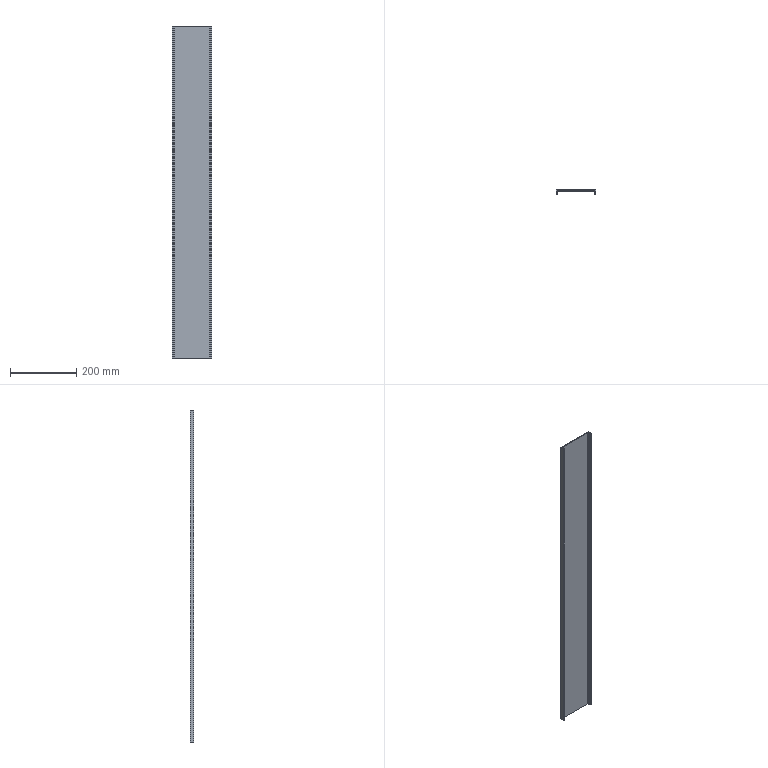Part | SolidWorks | features Extrusion 1, HoleWzd 1, ICE 1, MirrorPattern 1 | 1 solid | 48 faces | box 120 x 12 x 1000 mm | volume 423626 mm3 | cylinder 18 | plane 18 | cone 12 | commonest cylinder face diameters 2.6 x12 2.5 x6
STEP:
#1=CARTESIAN_POINT('',(-54.7,7.7,-480.));
#2=VERTEX_POINT('',#1);
#3=CARTESIAN_POINT('',(-54.735,7.4,-480.));
#4=VERTEX_POINT('',#3);
#5=CARTESIAN_POINT('',(-56.,7.7,-480.));
#6=DIRECTION('',(0.,0.,-1.));
#7=DIRECTION('',(-1.,0.,0.));
#8=AXIS2_PLACEMENT_3D('',#5,#6,#7);
#9=CIRCLE('',#8,1.3);
#10=EDGE_CURVE('',#2,#4,#9,.T.);
#11=ORIENTED_EDGE('',*,*,#10,.F.);
#12=CARTESIAN_POINT('',(-54.7,7.7,-500.));
#13=VERTEX_POINT('',#12);
#14=CARTESIAN_POINT('',(-54.7,7.7,-500.));
#15=DIRECTION('',(0.,0.,-1.));
#16=VECTOR('',#15,1000.);
#17=LINE('',#14,#16);
#18=EDGE_CURVE('',#2,#13,#17,.T.);
#19=ORIENTED_EDGE('',*,*,#18,.T.);
#20=CARTESIAN_POINT('',(-54.735,7.4,-500.));
#21=VERTEX_POINT('',#20);
#22=CARTESIAN_POINT('',(-56.,7.7,-500.));
#23=DIRECTION('',(0.,0.,-1.));
#24=DIRECTION('',(-1.,0.,0.));
#25=AXIS2_PLACEMENT_3D('',#22,#23,#24);
#26=CIRCLE('',#25,1.3);
#27=EDGE_CURVE('',#13,#21,#26,.T.);
#28=ORIENTED_EDGE('',*,*,#27,.T.);
#29=CARTESIAN_POINT('',(-54.735,7.4,-500.));
#30=DIRECTION('',(0.,0.,1.));
#31=VECTOR('',#30,1000.);
#32=LINE('',#29,#31);
#33=EDGE_CURVE('',#21,#4,#32,.T.);
#34=ORIENTED_EDGE('',*,*,#33,.T.);
#35=EDGE_LOOP('',(#11,#19,#28,#34));
#36=FACE_OUTER_BOUND('',#35,.T.);
#37=CARTESIAN_POINT('',(-56.,7.7,-500.));
#38=DIRECTION('',(0.,0.,-1.));
#39=DIRECTION('',(-1.,0.,0.));
#40=AXIS2_PLACEMENT_3D('',#37,#38,#39);
#41=CYLINDRICAL_SURFACE('',#40,1.3);
#42=ADVANCED_FACE('',(#36),#41,.F.);
#43=ORIENTED_EDGE('',*,*,#18,.F.);
#44=CARTESIAN_POINT('',(-57.3,7.7,-480.));
#45=VERTEX_POINT('',#44);
#46=CARTESIAN_POINT('',(-56.,7.7,-480.));
#47=DIRECTION('',(0.,0.,-1.));
#48=DIRECTION('',(-1.,0.,0.));
#49=AXIS2_PLACEMENT_3D('',#46,#47,#48);
#50=CIRCLE('',#49,1.3);
#51=EDGE_CURVE('',#45,#2,#50,.T.);
#52=ORIENTED_EDGE('',*,*,#51,.F.);
#53=CARTESIAN_POINT('',(-57.3,7.7,-500.));
#54=VERTEX_POINT('',#53);
#55=CARTESIAN_POINT('',(-57.3,7.7,-500.));
#56=DIRECTION('',(0.,0.,-1.));
#57=VECTOR('',#56,1000.);
#58=LINE('',#55,#57);
#59=EDGE_CURVE('',#45,#54,#58,.T.);
#60=ORIENTED_EDGE('',*,*,#59,.T.);
#61=CARTESIAN_POINT('',(-56.,7.7,-500.));
#62=DIRECTION('',(0.,0.,-1.));
#63=DIRECTION('',(-1.,0.,0.));
#64=AXIS2_PLACEMENT_3D('',#61,#62,#63);
#65=CIRCLE('',#64,1.3);
#66=EDGE_CURVE('',#54,#13,#65,.T.);
#67=ORIENTED_EDGE('',*,*,#66,.T.);
#68=EDGE_LOOP('',(#43,#52,#60,#67));
#69=FACE_OUTER_BOUND('',#68,.T.);
#70=CARTESIAN_POINT('',(-56.,7.7,-500.));
#71=DIRECTION('',(0.,0.,-1.));
#72=DIRECTION('',(-1.,0.,0.));
#73=AXIS2_PLACEMENT_3D('',#70,#71,#72);
#74=CYLINDRICAL_SURFACE('',#73,1.3);
#75=ADVANCED_FACE('',(#69),#74,.F.);
#76=CARTESIAN_POINT('',(-54.787,7.4,-479.97));
#77=VERTEX_POINT('',#76);
#78=CARTESIAN_POINT('',(-54.75,7.7,-479.97));
#79=VERTEX_POINT('',#78);
#80=CARTESIAN_POINT('',(-56.,7.7,-479.97));
#81=DIRECTION('',(0.,0.,1.));
#82=DIRECTION('',(-1.,0.,0.));
#83=AXIS2_PLACEMENT_3D('',#80,#81,#82);
#84=CIRCLE('',#83,1.25);
#85=EDGE_CURVE('',#77,#79,#84,.T.);
#86=ORIENTED_EDGE('',*,*,#85,.T.);
#87=CARTESIAN_POINT('',(-54.7,7.7,-480.));
#88=DIRECTION('',(0.8572,0.,-0.515));
#89=VECTOR('',#88,1000.);
#90=LINE('',#87,#89);
#91=EDGE_CURVE('',#79,#2,#90,.T.);
#92=ORIENTED_EDGE('',*,*,#91,.T.);
#93=ORIENTED_EDGE('',*,*,#10,.T.);
#94=CARTESIAN_POINT('',(-54.735,7.4,-480.));
#95=CARTESIAN_POINT('',(-54.752,7.4,-479.99));
#96=CARTESIAN_POINT('',(-54.769,7.4,-479.98));
#97=CARTESIAN_POINT('',(-54.787,7.4,-479.97));
#98=B_SPLINE_CURVE_WITH_KNOTS('',3,(#94,#95,#96,#97),.UNSPECIFIED.,.F.,.F.,(4,4),(0.001374,0.001433),.UNSPECIFIED.);
#99=EDGE_CURVE('',#4,#77,#98,.T.);
#100=ORIENTED_EDGE('',*,*,#99,.T.);
#101=EDGE_LOOP('',(#86,#92,#93,#100));
#102=FACE_OUTER_BOUND('',#101,.T.);
#103=CARTESIAN_POINT('',(-56.,7.7,-480.));
#104=DIRECTION('',(0.,0.,-1.));
#105=DIRECTION('',(-1.,0.,0.));
#106=AXIS2_PLACEMENT_3D('',#103,#104,#105);
#107=CONICAL_SURFACE('',#106,1.3,1.03);
#108=ADVANCED_FACE('',(#102),#107,.F.);
#109=ORIENTED_EDGE('',*,*,#91,.F.);
#110=CARTESIAN_POINT('',(-57.25,7.7,-479.97));
#111=VERTEX_POINT('',#110);
#112=CARTESIAN_POINT('',(-56.,7.7,-479.97));
#113=DIRECTION('',(0.,0.,1.));
#114=DIRECTION('',(-1.,0.,0.));
#115=AXIS2_PLACEMENT_3D('',#112,#113,#114);
#116=CIRCLE('',#115,1.25);
#117=EDGE_CURVE('',#79,#111,#116,.T.);
#118=ORIENTED_EDGE('',*,*,#117,.T.);
#119=CARTESIAN_POINT('',(-57.3,7.7,-480.));
#120=DIRECTION('',(-0.8572,0.,-0.515));
#121=VECTOR('',#120,1000.);
#122=LINE('',#119,#121);
#123=EDGE_CURVE('',#111,#45,#122,.T.);
#124=ORIENTED_EDGE('',*,*,#123,.T.);
#125=ORIENTED_EDGE('',*,*,#51,.T.);
#126=EDGE_LOOP('',(#109,#118,#124,#125));
#127=FACE_OUTER_BOUND('',#126,.T.);
#128=CARTESIAN_POINT('',(-56.,7.7,-480.));
#129=DIRECTION('',(0.,0.,-1.));
#130=DIRECTION('',(-1.,0.,0.));
#131=AXIS2_PLACEMENT_3D('',#128,#129,#130);
#132=CONICAL_SURFACE('',#131,1.3,1.03);
#133=ADVANCED_FACE('',(#127),#132,.F.);
#134=CARTESIAN_POINT('',(57.3,7.7,-480.));
#135=VERTEX_POINT('',#134);
#136=CARTESIAN_POINT('',(55.4,6.547,-480.));
#137=VERTEX_POINT('',#136);
#138=CARTESIAN_POINT('',(56.,7.7,-480.));
#139=DIRECTION('',(0.,0.,-1.));
#140=DIRECTION('',(-1.,0.,0.));
#141=AXIS2_PLACEMENT_3D('',#138,#139,#140);
#142=CIRCLE('',#141,1.3);
#143=EDGE_CURVE('',#135,#137,#142,.T.);
#144=ORIENTED_EDGE('',*,*,#143,.F.);
#145=CARTESIAN_POINT('',(57.3,7.7,-500.));
#146=VERTEX_POINT('',#145);
#147=CARTESIAN_POINT('',(57.3,7.7,-500.));
#148=DIRECTION('',(0.,0.,-1.));
#149=VECTOR('',#148,1000.);
#150=LINE('',#147,#149);
#151=EDGE_CURVE('',#135,#146,#150,.T.);
#152=ORIENTED_EDGE('',*,*,#151,.T.);
#153=CARTESIAN_POINT('',(55.4,6.547,-500.));
#154=VERTEX_POINT('',#153);
#155=CARTESIAN_POINT('',(56.,7.7,-500.));
#156=DIRECTION('',(0.,0.,-1.));
#157=DIRECTION('',(-1.,0.,0.));
#158=AXIS2_PLACEMENT_3D('',#155,#156,#157);
#159=CIRCLE('',#158,1.3);
#160=EDGE_CURVE('',#146,#154,#159,.T.);
#161=ORIENTED_EDGE('',*,*,#160,.T.);
#162=CARTESIAN_POINT('',(55.4,6.547,-500.));
#163=DIRECTION('',(0.,0.,1.));
#164=VECTOR('',#163,1000.);
#165=LINE('',#162,#164);
#166=EDGE_CURVE('',#154,#137,#165,.T.);
#167=ORIENTED_EDGE('',*,*,#166,.T.);
#168=EDGE_LOOP('',(#144,#152,#161,#167));
#169=FACE_OUTER_BOUND('',#168,.T.);
#170=CARTESIAN_POINT('',(56.,7.7,-500.));
#171=DIRECTION('',(0.,0.,-1.));
#172=DIRECTION('',(-1.,0.,0.));
#173=AXIS2_PLACEMENT_3D('',#170,#171,#172);
#174=CYLINDRICAL_SURFACE('',#173,1.3);
#175=ADVANCED_FACE('',(#169),#174,.F.);
#176=ORIENTED_EDGE('',*,*,#151,.F.);
#177=CARTESIAN_POINT('',(54.7,7.7,-480.));
#178=VERTEX_POINT('',#177);
#179=CARTESIAN_POINT('',(56.,7.7,-480.));
#180=DIRECTION('',(0.,0.,-1.));
#181=DIRECTION('',(-1.,0.,0.));
#182=AXIS2_PLACEMENT_3D('',#179,#180,#181);
#183=CIRCLE('',#182,1.3);
#184=EDGE_CURVE('',#178,#135,#183,.T.);
#185=ORIENTED_EDGE('',*,*,#184,.F.);
#186=CARTESIAN_POINT('',(54.7,7.7,-500.));
#187=VERTEX_POINT('',#186);
#188=CARTESIAN_POINT('',(54.7,7.7,-500.));
#189=DIRECTION('',(0.,0.,-1.));
#190=VECTOR('',#189,1000.);
#191=LINE('',#188,#190);
#192=EDGE_CURVE('',#178,#187,#191,.T.);
#193=ORIENTED_EDGE('',*,*,#192,.T.);
#194=CARTESIAN_POINT('',(56.,7.7,-500.));
#195=DIRECTION('',(0.,0.,-1.));
#196=DIRECTION('',(-1.,0.,0.));
#197=AXIS2_PLACEMENT_3D('',#194,#195,#196);
#198=CIRCLE('',#197,1.3);
#199=EDGE_CURVE('',#187,#146,#198,.T.);
#200=ORIENTED_EDGE('',*,*,#199,.T.);
#201=EDGE_LOOP('',(#176,#185,#193,#200));
#202=FACE_OUTER_BOUND('',#201,.T.);
#203=CARTESIAN_POINT('',(56.,7.7,-500.));
#204=DIRECTION('',(0.,0.,-1.));
#205=DIRECTION('',(-1.,0.,0.));
#206=AXIS2_PLACEMENT_3D('',#203,#204,#205);
#207=CYLINDRICAL_SURFACE('',#206,1.3);
#208=ADVANCED_FACE('',(#202),#207,.F.);
#209=CARTESIAN_POINT('',(55.4,6.603,-479.97));
#210=VERTEX_POINT('',#209);
#211=CARTESIAN_POINT('',(57.25,7.7,-479.97));
#212=VERTEX_POINT('',#211);
#213=CARTESIAN_POINT('',(56.,7.7,-479.97));
#214=DIRECTION('',(0.,0.,1.));
#215=DIRECTION('',(-1.,0.,0.));
#216=AXIS2_PLACEMENT_3D('',#213,#214,#215);
#217=CIRCLE('',#216,1.25);
#218=EDGE_CURVE('',#210,#212,#217,.T.);
#219=ORIENTED_EDGE('',*,*,#218,.T.);
#220=CARTESIAN_POINT('',(57.3,7.7,-480.));
#221=DIRECTION('',(0.8572,0.,-0.515));
#222=VECTOR('',#221,1000.);
#223=LINE('',#220,#222);
#224=EDGE_CURVE('',#212,#135,#223,.T.);
#225=ORIENTED_EDGE('',*,*,#224,.T.);
#226=ORIENTED_EDGE('',*,*,#143,.T.);
#227=CARTESIAN_POINT('',(55.4,6.547,-480.));
#228=CARTESIAN_POINT('',(55.4,6.566,-479.99));
#229=CARTESIAN_POINT('',(55.4,6.585,-479.98));
#230=CARTESIAN_POINT('',(55.4,6.603,-479.97));
#231=B_SPLINE_CURVE_WITH_KNOTS('',3,(#227,#228,#229,#230),.UNSPECIFIED.,.F.,.F.,(4,4),(0.001527,0.001591),.UNSPECIFIED.);
#232=EDGE_CURVE('',#137,#210,#231,.T.);
#233=ORIENTED_EDGE('',*,*,#232,.T.);
#234=EDGE_LOOP('',(#219,#225,#226,#233));
#235=FACE_OUTER_BOUND('',#234,.T.);
#236=CARTESIAN_POINT('',(56.,7.7,-480.));
#237=DIRECTION('',(0.,0.,-1.));
#238=DIRECTION('',(-1.,0.,0.));
#239=AXIS2_PLACEMENT_3D('',#236,#237,#238);
#240=CONICAL_SURFACE('',#239,1.3,1.03);
#241=ADVANCED_FACE('',(#235),#240,.F.);
#242=ORIENTED_EDGE('',*,*,#224,.F.);
#243=CARTESIAN_POINT('',(54.75,7.7,-479.97));
#244=VERTEX_POINT('',#243);
#245=CARTESIAN_POINT('',(56.,7.7,-479.97));
#246=DIRECTION('',(0.,0.,1.));
#247=DIRECTION('',(-1.,0.,0.));
#248=AXIS2_PLACEMENT_3D('',#245,#246,#247);
#249=CIRCLE('',#248,1.25);
#250=EDGE_CURVE('',#212,#244,#249,.T.);
#251=ORIENTED_EDGE('',*,*,#250,.T.);
#252=CARTESIAN_POINT('',(54.7,7.7,-480.));
#253=DIRECTION('',(-0.8572,0.,-0.515));
#254=VECTOR('',#253,1000.);
#255=LINE('',#252,#254);
#256=EDGE_CURVE('',#244,#178,#255,.T.);
#257=ORIENTED_EDGE('',*,*,#256,.T.);
#258=ORIENTED_EDGE('',*,*,#184,.T.);
#259=EDGE_LOOP('',(#242,#251,#257,#258));
#260=FACE_OUTER_BOUND('',#259,.T.);
#261=CARTESIAN_POINT('',(56.,7.7,-480.));
#262=DIRECTION('',(0.,0.,-1.));
#263=DIRECTION('',(-1.,0.,0.));
#264=AXIS2_PLACEMENT_3D('',#261,#262,#263);
#265=CONICAL_SURFACE('',#264,1.3,1.03);
#266=ADVANCED_FACE('',(#260),#265,.F.);
#267=CARTESIAN_POINT('',(-57.3,7.7,480.));
#268=VERTEX_POINT('',#267);
#269=CARTESIAN_POINT('',(-55.4,6.547,480.));
#270=VERTEX_POINT('',#269);
#271=CARTESIAN_POINT('',(-56.,7.7,480.));
#272=DIRECTION('',(0.,0.,1.));
#273=DIRECTION('',(1.,0.,0.));
#274=AXIS2_PLACEMENT_3D('',#271,#272,#273);
#275=CIRCLE('',#274,1.3);
#276=EDGE_CURVE('',#268,#270,#275,.T.);
#277=ORIENTED_EDGE('',*,*,#276,.F.);
#278=CARTESIAN_POINT('',(-57.3,7.7,500.));
#279=VERTEX_POINT('',#278);
#280=CARTESIAN_POINT('',(-57.3,7.7,500.));
#281=DIRECTION('',(0.,0.,1.));
#282=VECTOR('',#281,1000.);
#283=LINE('',#280,#282);
#284=EDGE_CURVE('',#268,#279,#283,.T.);
#285=ORIENTED_EDGE('',*,*,#284,.T.);
#286=CARTESIAN_POINT('',(-55.4,6.547,500.));
#287=VERTEX_POINT('',#286);
#288=CARTESIAN_POINT('',(-56.,7.7,500.));
#289=DIRECTION('',(0.,0.,1.));
#290=DIRECTION('',(1.,0.,0.));
#291=AXIS2_PLACEMENT_3D('',#288,#289,#290);
#292=CIRCLE('',#291,1.3);
#293=EDGE_CURVE('',#279,#287,#292,.T.);
#294=ORIENTED_EDGE('',*,*,#293,.T.);
#295=CARTESIAN_POINT('',(-55.4,6.547,500.));
#296=DIRECTION('',(0.,0.,-1.));
#297=VECTOR('',#296,1000.);
#298=LINE('',#295,#297);
#299=EDGE_CURVE('',#287,#270,#298,.T.);
#300=ORIENTED_EDGE('',*,*,#299,.T.);
#301=EDGE_LOOP('',(#277,#285,#294,#300));
#302=FACE_OUTER_BOUND('',#301,.T.);
#303=CARTESIAN_POINT('',(-56.,7.7,500.));
#304=DIRECTION('',(0.,0.,1.));
#305=DIRECTION('',(1.,0.,0.));
#306=AXIS2_PLACEMENT_3D('',#303,#304,#305);
#307=CYLINDRICAL_SURFACE('',#306,1.3);
#308=ADVANCED_FACE('',(#302),#307,.F.);
#309=ORIENTED_EDGE('',*,*,#284,.F.);
#310=CARTESIAN_POINT('',(-54.7,7.7,480.));
#311=VERTEX_POINT('',#310);
#312=CARTESIAN_POINT('',(-56.,7.7,480.));
#313=DIRECTION('',(0.,0.,1.));
#314=DIRECTION('',(1.,0.,0.));
#315=AXIS2_PLACEMENT_3D('',#312,#313,#314);
#316=CIRCLE('',#315,1.3);
#317=EDGE_CURVE('',#311,#268,#316,.T.);
#318=ORIENTED_EDGE('',*,*,#317,.F.);
#319=CARTESIAN_POINT('',(-54.7,7.7,500.));
#320=VERTEX_POINT('',#319);
#321=CARTESIAN_POINT('',(-54.7,7.7,500.));
#322=DIRECTION('',(0.,0.,1.));
#323=VECTOR('',#322,1000.);
#324=LINE('',#321,#323);
#325=EDGE_CURVE('',#311,#320,#324,.T.);
#326=ORIENTED_EDGE('',*,*,#325,.T.);
#327=CARTESIAN_POINT('',(-56.,7.7,500.));
#328=DIRECTION('',(0.,0.,1.));
#329=DIRECTION('',(1.,0.,0.));
#330=AXIS2_PLACEMENT_3D('',#327,#328,#329);
#331=CIRCLE('',#330,1.3);
#332=EDGE_CURVE('',#320,#279,#331,.T.);
#333=ORIENTED_EDGE('',*,*,#332,.T.);
#334=EDGE_LOOP('',(#309,#318,#326,#333));
#335=FACE_OUTER_BOUND('',#334,.T.);
#336=CARTESIAN_POINT('',(-56.,7.7,500.));
#337=DIRECTION('',(0.,0.,1.));
#338=DIRECTION('',(1.,0.,0.));
#339=AXIS2_PLACEMENT_3D('',#336,#337,#338);
#340=CYLINDRICAL_SURFACE('',#339,1.3);
#341=ADVANCED_FACE('',(#335),#340,.F.);
#342=CARTESIAN_POINT('',(-55.4,6.603,479.97));
#343=VERTEX_POINT('',#342);
#344=CARTESIAN_POINT('',(-57.25,7.7,479.97));
#345=VERTEX_POINT('',#344);
#346=CARTESIAN_POINT('',(-56.,7.7,479.97));
#347=DIRECTION('',(0.,0.,-1.));
#348=DIRECTION('',(1.,0.,0.));
#349=AXIS2_PLACEMENT_3D('',#346,#347,#348);
#350=CIRCLE('',#349,1.25);
#351=EDGE_CURVE('',#343,#345,#350,.T.);
#352=ORIENTED_EDGE('',*,*,#351,.T.);
#353=CARTESIAN_POINT('',(-57.3,7.7,480.));
#354=DIRECTION('',(-0.8572,0.,0.515));
#355=VECTOR('',#354,1000.);
#356=LINE('',#353,#355);
#357=EDGE_CURVE('',#345,#268,#356,.T.);
#358=ORIENTED_EDGE('',*,*,#357,.T.);
#359=ORIENTED_EDGE('',*,*,#276,.T.);
#360=CARTESIAN_POINT('',(-55.4,6.547,480.));
#361=CARTESIAN_POINT('',(-55.4,6.566,479.99));
#362=CARTESIAN_POINT('',(-55.4,6.585,479.98));
#363=CARTESIAN_POINT('',(-55.4,6.603,479.97));
#364=B_SPLINE_CURVE_WITH_KNOTS('',3,(#360,#361,#362,#363),.UNSPECIFIED.,.F.,.F.,(4,4),(0.001527,0.001591),.UNSPECIFIED.);
#365=EDGE_CURVE('',#270,#343,#364,.T.);
#366=ORIENTED_EDGE('',*,*,#365,.T.);
#367=EDGE_LOOP('',(#352,#358,#359,#366));
#368=FACE_OUTER_BOUND('',#367,.T.);
#369=CARTESIAN_POINT('',(-56.,7.7,480.));
#370=DIRECTION('',(0.,0.,1.));
#371=DIRECTION('',(1.,0.,0.));
#372=AXIS2_PLACEMENT_3D('',#369,#370,#371);
#373=CONICAL_SURFACE('',#372,1.3,1.03);
#374=ADVANCED_FACE('',(#368),#373,.F.);
#375=ORIENTED_EDGE('',*,*,#357,.F.);
#376=CARTESIAN_POINT('',(-54.75,7.7,479.97));
#377=VERTEX_POINT('',#376);
#378=CARTESIAN_POINT('',(-56.,7.7,479.97));
#379=DIRECTION('',(0.,0.,-1.));
#380=DIRECTION('',(1.,0.,0.));
#381=AXIS2_PLACEMENT_3D('',#378,#379,#380);
#382=CIRCLE('',#381,1.25);
#383=EDGE_CURVE('',#345,#377,#382,.T.);
#384=ORIENTED_EDGE('',*,*,#383,.T.);
#385=CARTESIAN_POINT('',(-54.7,7.7,480.));
#386=DIRECTION('',(0.8572,0.,0.515));
#387=VECTOR('',#386,1000.);
#388=LINE('',#385,#387);
#389=EDGE_CURVE('',#377,#311,#388,.T.);
#390=ORIENTED_EDGE('',*,*,#389,.T.);
#391=ORIENTED_EDGE('',*,*,#317,.T.);
#392=EDGE_LOOP('',(#375,#384,#390,#391));
#393=FACE_OUTER_BOUND('',#392,.T.);
#394=CARTESIAN_POINT('',(-56.,7.7,480.));
#395=DIRECTION('',(0.,0.,1.));
#396=DIRECTION('',(1.,0.,0.));
#397=AXIS2_PLACEMENT_3D('',#394,#395,#396);
#398=CONICAL_SURFACE('',#397,1.3,1.03);
#399=ADVANCED_FACE('',(#393),#398,.F.);
#400=CARTESIAN_POINT('',(54.7,7.7,480.));
#401=VERTEX_POINT('',#400);
#402=CARTESIAN_POINT('',(54.735,7.4,480.));
#403=VERTEX_POINT('',#402);
#404=CARTESIAN_POINT('',(56.,7.7,480.));
#405=DIRECTION('',(0.,0.,1.));
#406=DIRECTION('',(1.,0.,0.));
#407=AXIS2_PLACEMENT_3D('',#404,#405,#406);
#408=CIRCLE('',#407,1.3);
#409=EDGE_CURVE('',#401,#403,#408,.T.);
#410=ORIENTED_EDGE('',*,*,#409,.F.);
#411=CARTESIAN_POINT('',(54.7,7.7,500.));
#412=VERTEX_POINT('',#411);
#413=CARTESIAN_POINT('',(54.7,7.7,500.));
#414=DIRECTION('',(0.,0.,1.));
#415=VECTOR('',#414,1000.);
#416=LINE('',#413,#415);
#417=EDGE_CURVE('',#401,#412,#416,.T.);
#418=ORIENTED_EDGE('',*,*,#417,.T.);
#419=CARTESIAN_POINT('',(54.735,7.4,500.));
#420=VERTEX_POINT('',#419);
#421=CARTESIAN_POINT('',(56.,7.7,500.));
#422=DIRECTION('',(0.,0.,-1.));
#423=DIRECTION('',(-1.,0.,0.));
#424=AXIS2_PLACEMENT_3D('',#421,#422,#423);
#425=CIRCLE('',#424,1.3);
#426=EDGE_CURVE('',#420,#412,#425,.T.);
#427=ORIENTED_EDGE('',*,*,#426,.F.);
#428=CARTESIAN_POINT('',(54.735,7.4,500.));
#429=DIRECTION('',(0.,0.,-1.));
#430=VECTOR('',#429,1000.);
#431=LINE('',#428,#430);
#432=EDGE_CURVE('',#420,#403,#431,.T.);
#433=ORIENTED_EDGE('',*,*,#432,.T.);
#434=EDGE_LOOP('',(#410,#418,#427,#433));
#435=FACE_OUTER_BOUND('',#434,.T.);
#436=CARTESIAN_POINT('',(56.,7.7,500.));
#437=DIRECTION('',(0.,0.,1.));
#438=DIRECTION('',(1.,0.,0.));
#439=AXIS2_PLACEMENT_3D('',#436,#437,#438);
#440=CYLINDRICAL_SURFACE('',#439,1.3);
#441=ADVANCED_FACE('',(#435),#440,.F.);
#442=ORIENTED_EDGE('',*,*,#417,.F.);
#443=CARTESIAN_POINT('',(57.3,7.7,480.));
#444=VERTEX_POINT('',#443);
#445=CARTESIAN_POINT('',(56.,7.7,480.));
#446=DIRECTION('',(0.,0.,1.));
#447=DIRECTION('',(1.,0.,0.));
#448=AXIS2_PLACEMENT_3D('',#445,#446,#447);
#449=CIRCLE('',#448,1.3);
#450=EDGE_CURVE('',#444,#401,#449,.T.);
#451=ORIENTED_EDGE('',*,*,#450,.F.);
#452=CARTESIAN_POINT('',(57.3,7.7,500.));
#453=VERTEX_POINT('',#452);
#454=CARTESIAN_POINT('',(57.3,7.7,500.));
#455=DIRECTION('',(0.,0.,1.));
#456=VECTOR('',#455,1000.);
#457=LINE('',#454,#456);
#458=EDGE_CURVE('',#444,#453,#457,.T.);
#459=ORIENTED_EDGE('',*,*,#458,.T.);
#460=CARTESIAN_POINT('',(56.,7.7,500.));
#461=DIRECTION('',(0.,0.,-1.));
#462=DIRECTION('',(-1.,0.,0.));
#463=AXIS2_PLACEMENT_3D('',#460,#461,#462);
#464=CIRCLE('',#463,1.3);
#465=EDGE_CURVE('',#412,#453,#464,.T.);
#466=ORIENTED_EDGE('',*,*,#465,.F.);
#467=EDGE_LOOP('',(#442,#451,#459,#466));
#468=FACE_OUTER_BOUND('',#467,.T.);
#469=CARTESIAN_POINT('',(56.,7.7,500.));
#470=DIRECTION('',(0.,0.,1.));
#471=DIRECTION('',(1.,0.,0.));
#472=AXIS2_PLACEMENT_3D('',#469,#470,#471);
#473=CYLINDRICAL_SURFACE('',#472,1.3);
#474=ADVANCED_FACE('',(#468),#473,.F.);
#475=CARTESIAN_POINT('',(54.787,7.4,479.97));
#476=VERTEX_POINT('',#475);
#477=CARTESIAN_POINT('',(54.75,7.7,479.97));
#478=VERTEX_POINT('',#477);
#479=CARTESIAN_POINT('',(56.,7.7,479.97));
#480=DIRECTION('',(0.,0.,-1.));
#481=DIRECTION('',(1.,0.,0.));
#482=AXIS2_PLACEMENT_3D('',#479,#480,#481);
#483=CIRCLE('',#482,1.25);
#484=EDGE_CURVE('',#476,#478,#483,.T.);
#485=ORIENTED_EDGE('',*,*,#484,.T.);
#486=CARTESIAN_POINT('',(54.7,7.7,480.));
#487=DIRECTION('',(-0.8572,0.,0.515));
#488=VECTOR('',#487,1000.);
#489=LINE('',#486,#488);
#490=EDGE_CURVE('',#478,#401,#489,.T.);
#491=ORIENTED_EDGE('',*,*,#490,.T.);
#492=ORIENTED_EDGE('',*,*,#409,.T.);
#493=CARTESIAN_POINT('',(54.735,7.4,480.));
#494=CARTESIAN_POINT('',(54.752,7.4,479.99));
#495=CARTESIAN_POINT('',(54.769,7.4,479.98));
#496=CARTESIAN_POINT('',(54.787,7.4,479.97));
#497=B_SPLINE_CURVE_WITH_KNOTS('',3,(#493,#494,#495,#496),.UNSPECIFIED.,.F.,.F.,(4,4),(0.001374,0.001433),.UNSPECIFIED.);
#498=EDGE_CURVE('',#403,#476,#497,.T.);
#499=ORIENTED_EDGE('',*,*,#498,.T.);
#500=EDGE_LOOP('',(#485,#491,#492,#499));
#501=FACE_OUTER_BOUND('',#500,.T.);
#502=CARTESIAN_POINT('',(56.,7.7,480.));
#503=DIRECTION('',(0.,0.,1.));
#504=DIRECTION('',(1.,0.,0.));
#505=AXIS2_PLACEMENT_3D('',#502,#503,#504);
#506=CONICAL_SURFACE('',#505,1.3,1.03);
#507=ADVANCED_FACE('',(#501),#506,.F.);
#508=ORIENTED_EDGE('',*,*,#490,.F.);
#509=CARTESIAN_POINT('',(57.25,7.7,479.97));
#510=VERTEX_POINT('',#509);
#511=CARTESIAN_POINT('',(56.,7.7,479.97));
#512=DIRECTION('',(0.,0.,-1.));
#513=DIRECTION('',(1.,0.,0.));
#514=AXIS2_PLACEMENT_3D('',#511,#512,#513);
#515=CIRCLE('',#514,1.25);
#516=EDGE_CURVE('',#478,#510,#515,.T.);
#517=ORIENTED_EDGE('',*,*,#516,.T.);
#518=CARTESIAN_POINT('',(57.3,7.7,480.));
#519=DIRECTION('',(0.8572,0.,0.515));
#520=VECTOR('',#519,1000.);
#521=LINE('',#518,#520);
#522=EDGE_CURVE('',#510,#444,#521,.T.);
#523=ORIENTED_EDGE('',*,*,#522,.T.);
#524=ORIENTED_EDGE('',*,*,#450,.T.);
#525=EDGE_LOOP('',(#508,#517,#523,#524));
#526=FACE_OUTER_BOUND('',#525,.T.);
#527=CARTESIAN_POINT('',(56.,7.7,480.));
#528=DIRECTION('',(0.,0.,1.));
#529=DIRECTION('',(1.,0.,0.));
#530=AXIS2_PLACEMENT_3D('',#527,#528,#529);
#531=CONICAL_SURFACE('',#530,1.3,1.03);
#532=ADVANCED_FACE('',(#526),#531,.F.);
#533=CARTESIAN_POINT('',(-54.787,7.4,479.97));
#534=VERTEX_POINT('',#533);
#535=CARTESIAN_POINT('',(-56.,7.7,479.97));
#536=DIRECTION('',(0.,0.,-1.));
#537=DIRECTION('',(1.,0.,0.));
#538=AXIS2_PLACEMENT_3D('',#535,#536,#537);
#539=CIRCLE('',#538,1.25);
#540=EDGE_CURVE('',#377,#534,#539,.T.);
#541=ORIENTED_EDGE('',*,*,#540,.F.);
#542=CARTESIAN_POINT('',(-54.75,7.7,500.));
#543=DIRECTION('',(0.,0.,-1.));
#544=VECTOR('',#543,1000.);
#545=LINE('',#542,#544);
#546=EDGE_CURVE('',#377,#79,#545,.T.);
#547=ORIENTED_EDGE('',*,*,#546,.T.);
#548=ORIENTED_EDGE('',*,*,#85,.F.);
#549=CARTESIAN_POINT('',(-54.787,7.4,500.));
#550=DIRECTION('',(0.,0.,1.));
#551=VECTOR('',#550,1000.);
#552=LINE('',#549,#551);
#553=EDGE_CURVE('',#77,#534,#552,.T.);
#554=ORIENTED_EDGE('',*,*,#553,.T.);
#555=EDGE_LOOP('',(#541,#547,#548,#554));
#556=FACE_OUTER_BOUND('',#555,.T.);
#557=CARTESIAN_POINT('',(-56.,7.7,500.));
#558=DIRECTION('',(0.,0.,-1.));
#559=DIRECTION('',(-1.,0.,0.));
#560=AXIS2_PLACEMENT_3D('',#557,#558,#559);
#561=CYLINDRICAL_SURFACE('',#560,1.25);
#562=ADVANCED_FACE('',(#556),#561,.F.);
#563=ORIENTED_EDGE('',*,*,#546,.F.);
#564=ORIENTED_EDGE('',*,*,#383,.F.);
#565=CARTESIAN_POINT('',(-57.25,7.7,500.));
#566=DIRECTION('',(0.,0.,-1.));
#567=VECTOR('',#566,1000.);
#568=LINE('',#565,#567);
#569=EDGE_CURVE('',#345,#111,#568,.T.);
#570=ORIENTED_EDGE('',*,*,#569,.T.);
#571=ORIENTED_EDGE('',*,*,#117,.F.);
#572=EDGE_LOOP('',(#563,#564,#570,#571));
#573=FACE_OUTER_BOUND('',#572,.T.);
#574=CARTESIAN_POINT('',(-56.,7.7,500.));
#575=DIRECTION('',(0.,0.,-1.));
#576=DIRECTION('',(-1.,0.,0.));
#577=AXIS2_PLACEMENT_3D('',#574,#575,#576);
#578=CYLINDRICAL_SURFACE('',#577,1.25);
#579=ADVANCED_FACE('',(#573),#578,.F.);
#580=CARTESIAN_POINT('',(55.4,6.603,479.97));
#581=VERTEX_POINT('',#580);
#582=CARTESIAN_POINT('',(56.,7.7,479.97));
#583=DIRECTION('',(0.,0.,-1.));
#584=DIRECTION('',(1.,0.,0.));
#585=AXIS2_PLACEMENT_3D('',#582,#583,#584);
#586=CIRCLE('',#585,1.25);
#587=EDGE_CURVE('',#510,#581,#586,.T.);
#588=ORIENTED_EDGE('',*,*,#587,.F.);
#589=CARTESIAN_POINT('',(57.25,7.7,500.));
#590=DIRECTION('',(0.,0.,-1.));
#591=VECTOR('',#590,1000.);
#592=LINE('',#589,#591);
#593=EDGE_CURVE('',#510,#212,#592,.T.);
#594=ORIENTED_EDGE('',*,*,#593,.T.);
#595=ORIENTED_EDGE('',*,*,#218,.F.);
#596=CARTESIAN_POINT('',(55.4,6.603,500.));
#597=DIRECTION('',(0.,0.,1.));
#598=VECTOR('',#597,1000.);
#599=LINE('',#596,#598);
#600=EDGE_CURVE('',#210,#581,#599,.T.);
#601=ORIENTED_EDGE('',*,*,#600,.T.);
#602=EDGE_LOOP('',(#588,#594,#595,#601));
#603=FACE_OUTER_BOUND('',#602,.T.);
#604=CARTESIAN_POINT('',(56.,7.7,500.));
#605=DIRECTION('',(0.,0.,-1.));
#606=DIRECTION('',(-1.,0.,0.));
#607=AXIS2_PLACEMENT_3D('',#604,#605,#606);
#608=CYLINDRICAL_SURFACE('',#607,1.25);
#609=ADVANCED_FACE('',(#603),#608,.F.);
#610=ORIENTED_EDGE('',*,*,#593,.F.);
#611=ORIENTED_EDGE('',*,*,#516,.F.);
#612=CARTESIAN_POINT('',(54.75,7.7,500.));
#613=DIRECTION('',(0.,0.,-1.));
#614=VECTOR('',#613,1000.);
#615=LINE('',#612,#614);
#616=EDGE_CURVE('',#478,#244,#615,.T.);
#617=ORIENTED_EDGE('',*,*,#616,.T.);
#618=ORIENTED_EDGE('',*,*,#250,.F.);
#619=EDGE_LOOP('',(#610,#611,#617,#618));
#620=FACE_OUTER_BOUND('',#619,.T.);
#621=CARTESIAN_POINT('',(56.,7.7,500.));
#622=DIRECTION('',(0.,0.,-1.));
#623=DIRECTION('',(-1.,0.,0.));
#624=AXIS2_PLACEMENT_3D('',#621,#622,#623);
#625=CYLINDRICAL_SURFACE('',#624,1.25);
#626=ADVANCED_FACE('',(#620),#625,.F.);
#627=CARTESIAN_POINT('',(-54.735,7.4,500.));
#628=VERTEX_POINT('',#627);
#629=CARTESIAN_POINT('',(-56.,7.7,500.));
#630=DIRECTION('',(0.,0.,1.));
#631=DIRECTION('',(1.,0.,0.));
#632=AXIS2_PLACEMENT_3D('',#629,#630,#631);
#633=CIRCLE('',#632,1.3);
#634=EDGE_CURVE('',#628,#320,#633,.T.);
#635=ORIENTED_EDGE('',*,*,#634,.F.);
#636=CARTESIAN_POINT('',(-53.7,7.4,500.));
#637=VERTEX_POINT('',#636);
#638=CARTESIAN_POINT('',(-53.7,7.4,500.));
#639=DIRECTION('',(-1.,0.,0.));
#640=VECTOR('',#639,1000.);
#641=LINE('',#638,#640);
#642=EDGE_CURVE('',#637,#628,#641,.T.);
#643=ORIENTED_EDGE('',*,*,#642,.F.);
#644=CARTESIAN_POINT('',(-53.7,9.,500.));
#645=VERTEX_POINT('',#644);
#646=CARTESIAN_POINT('',(-53.7,5.5,500.));
#647=DIRECTION('',(0.,1.,0.));
#648=VECTOR('',#647,1000.);
#649=LINE('',#646,#648);
#650=EDGE_CURVE('',#637,#645,#649,.T.);
#651=ORIENTED_EDGE('',*,*,#650,.T.);
#652=CARTESIAN_POINT('',(53.7,9.,500.));
#653=VERTEX_POINT('',#652);
#654=CARTESIAN_POINT('',(-53.7,9.,500.));
#655=DIRECTION('',(1.,0.,0.));
#656=VECTOR('',#655,1000.);
#657=LINE('',#654,#656);
#658=EDGE_CURVE('',#645,#653,#657,.T.);
#659=ORIENTED_EDGE('',*,*,#658,.T.);
#660=CARTESIAN_POINT('',(53.7,7.4,500.));
#661=VERTEX_POINT('',#660);
#662=CARTESIAN_POINT('',(53.7,5.5,500.));
#663=DIRECTION('',(0.,-1.,0.));
#664=VECTOR('',#663,1000.);
#665=LINE('',#662,#664);
#666=EDGE_CURVE('',#653,#661,#665,.T.);
#667=ORIENTED_EDGE('',*,*,#666,.T.);
#668=CARTESIAN_POINT('',(53.7,7.4,500.));
#669=DIRECTION('',(-1.,0.,0.));
#670=VECTOR('',#669,1000.);
#671=LINE('',#668,#670);
#672=EDGE_CURVE('',#420,#661,#671,.T.);
#673=ORIENTED_EDGE('',*,*,#672,.F.);
#674=ORIENTED_EDGE('',*,*,#426,.T.);
#675=ORIENTED_EDGE('',*,*,#465,.T.);
#676=CARTESIAN_POINT('',(55.4,6.547,500.));
#677=VERTEX_POINT('',#676);
#678=CARTESIAN_POINT('',(56.,7.7,500.));
#679=DIRECTION('',(0.,0.,-1.));
#680=DIRECTION('',(-1.,0.,0.));
#681=AXIS2_PLACEMENT_3D('',#678,#679,#680);
#682=CIRCLE('',#681,1.3);
#683=EDGE_CURVE('',#453,#677,#682,.T.);
#684=ORIENTED_EDGE('',*,*,#683,.T.);
#685=CARTESIAN_POINT('',(55.4,5.5,500.));
#686=VERTEX_POINT('',#685);
#687=CARTESIAN_POINT('',(55.4,5.5,500.));
#688=DIRECTION('',(0.,1.,0.));
#689=VECTOR('',#688,1000.);
#690=LINE('',#687,#689);
#691=EDGE_CURVE('',#686,#677,#690,.T.);
#692=ORIENTED_EDGE('',*,*,#691,.F.);
#693=CARTESIAN_POINT('',(56.8,5.5,500.));
#694=VERTEX_POINT('',#693);
#695=CARTESIAN_POINT('',(56.8,5.5,500.));
#696=DIRECTION('',(1.,0.,0.));
#697=VECTOR('',#696,1000.);
#698=LINE('',#695,#697);
#699=EDGE_CURVE('',#686,#694,#698,.T.);
#700=ORIENTED_EDGE('',*,*,#699,.T.);
#701=CARTESIAN_POINT('',(56.8,0.,500.));
#702=VERTEX_POINT('',#701);
#703=CARTESIAN_POINT('',(56.8,0.,500.));
#704=DIRECTION('',(0.,-1.,0.));
#705=VECTOR('',#704,1000.);
#706=LINE('',#703,#705);
#707=EDGE_CURVE('',#694,#702,#706,.T.);
#708=ORIENTED_EDGE('',*,*,#707,.T.);
#709=CARTESIAN_POINT('',(60.,0.,500.));
#710=VERTEX_POINT('',#709);
#711=CARTESIAN_POINT('',(60.,0.,500.));
#712=DIRECTION('',(1.,0.,0.));
#713=VECTOR('',#712,1000.);
#714=LINE('',#711,#713);
#715=EDGE_CURVE('',#702,#710,#714,.T.);
#716=ORIENTED_EDGE('',*,*,#715,.T.);
#717=CARTESIAN_POINT('',(60.,12.,500.));
#718=VERTEX_POINT('',#717);
#719=CARTESIAN_POINT('',(60.,12.,500.));
#720=DIRECTION('',(0.,1.,0.));
#721=VECTOR('',#720,1000.);
#722=LINE('',#719,#721);
#723=EDGE_CURVE('',#710,#718,#722,.T.);
#724=ORIENTED_EDGE('',*,*,#723,.T.);
#725=CARTESIAN_POINT('',(-60.,12.,500.));
#726=VERTEX_POINT('',#725);
#727=CARTESIAN_POINT('',(60.,12.,500.));
#728=DIRECTION('',(-1.,0.,0.));
#729=VECTOR('',#728,1000.);
#730=LINE('',#727,#729);
#731=EDGE_CURVE('',#718,#726,#730,.T.);
#732=ORIENTED_EDGE('',*,*,#731,.T.);
#733=CARTESIAN_POINT('',(-60.,0.,500.));
#734=VERTEX_POINT('',#733);
#735=CARTESIAN_POINT('',(-60.,12.,500.));
#736=DIRECTION('',(0.,-1.,0.));
#737=VECTOR('',#736,1000.);
#738=LINE('',#735,#737);
#739=EDGE_CURVE('',#726,#734,#738,.T.);
#740=ORIENTED_EDGE('',*,*,#739,.T.);
#741=CARTESIAN_POINT('',(-56.8,0.,500.));
#742=VERTEX_POINT('',#741);
#743=CARTESIAN_POINT('',(-60.,0.,500.));
#744=DIRECTION('',(1.,0.,0.));
#745=VECTOR('',#744,1000.);
#746=LINE('',#743,#745);
#747=EDGE_CURVE('',#734,#742,#746,.T.);
#748=ORIENTED_EDGE('',*,*,#747,.T.);
#749=CARTESIAN_POINT('',(-56.8,5.5,500.));
#750=VERTEX_POINT('',#749);
#751=CARTESIAN_POINT('',(-56.8,0.,500.));
#752=DIRECTION('',(0.,1.,0.));
#753=VECTOR('',#752,1000.);
#754=LINE('',#751,#753);
#755=EDGE_CURVE('',#742,#750,#754,.T.);
#756=ORIENTED_EDGE('',*,*,#755,.T.);
#757=CARTESIAN_POINT('',(-55.4,5.5,500.));
#758=VERTEX_POINT('',#757);
#759=CARTESIAN_POINT('',(-56.8,5.5,500.));
#760=DIRECTION('',(1.,0.,0.));
#761=VECTOR('',#760,1000.);
#762=LINE('',#759,#761);
#763=EDGE_CURVE('',#750,#758,#762,.T.);
#764=ORIENTED_EDGE('',*,*,#763,.T.);
#765=CARTESIAN_POINT('',(-55.4,5.5,500.));
#766=DIRECTION('',(0.,-1.,0.));
#767=VECTOR('',#766,1000.);
#768=LINE('',#765,#767);
#769=EDGE_CURVE('',#287,#758,#768,.T.);
#770=ORIENTED_EDGE('',*,*,#769,.F.);
#771=ORIENTED_EDGE('',*,*,#293,.F.);
#772=ORIENTED_EDGE('',*,*,#332,.F.);
#773=EDGE_LOOP('',(#635,#643,#651,#659,#667,#673,#674,#675,#684,#692,#700,#708,#716,#724,#732,#740,#748,#756,#764,#770,#771,#772));
#774=FACE_OUTER_BOUND('',#773,.T.);
#775=CARTESIAN_POINT('',(0.,0.,500.));
#776=DIRECTION('',(0.,0.,-1.));
#777=DIRECTION('',(-1.,0.,0.));
#778=AXIS2_PLACEMENT_3D('',#775,#776,#777);
#779=PLANE('',#778);
#780=ADVANCED_FACE('',(#774),#779,.F.);
#781=CARTESIAN_POINT('',(-55.4,6.547,-500.));
#782=VERTEX_POINT('',#781);
#783=CARTESIAN_POINT('',(-56.,7.7,-500.));
#784=DIRECTION('',(0.,0.,-1.));
#785=DIRECTION('',(-1.,0.,0.));
#786=AXIS2_PLACEMENT_3D('',#783,#784,#785);
#787=CIRCLE('',#786,1.3);
#788=EDGE_CURVE('',#782,#54,#787,.T.);
#789=ORIENTED_EDGE('',*,*,#788,.F.);
#790=CARTESIAN_POINT('',(-55.4,5.5,-500.));
#791=VERTEX_POINT('',#790);
#792=CARTESIAN_POINT('',(-55.4,5.5,-500.));
#793=DIRECTION('',(0.,-1.,0.));
#794=VECTOR('',#793,1000.);
#795=LINE('',#792,#794);
#796=EDGE_CURVE('',#782,#791,#795,.T.);
#797=ORIENTED_EDGE('',*,*,#796,.T.);
#798=CARTESIAN_POINT('',(-56.8,5.5,-500.));
#799=VERTEX_POINT('',#798);
#800=CARTESIAN_POINT('',(-56.8,5.5,-500.));
#801=DIRECTION('',(1.,0.,0.));
#802=VECTOR('',#801,1000.);
#803=LINE('',#800,#802);
#804=EDGE_CURVE('',#799,#791,#803,.T.);
#805=ORIENTED_EDGE('',*,*,#804,.F.);
#806=CARTESIAN_POINT('',(-56.8,0.,-500.));
#807=VERTEX_POINT('',#806);
#808=CARTESIAN_POINT('',(-56.8,0.,-500.));
#809=DIRECTION('',(0.,1.,0.));
#810=VECTOR('',#809,1000.);
#811=LINE('',#808,#810);
#812=EDGE_CURVE('',#807,#799,#811,.T.);
#813=ORIENTED_EDGE('',*,*,#812,.F.);
#814=CARTESIAN_POINT('',(-60.,0.,-500.));
#815=VERTEX_POINT('',#814);
#816=CARTESIAN_POINT('',(-60.,0.,-500.));
#817=DIRECTION('',(1.,0.,0.));
#818=VECTOR('',#817,1000.);
#819=LINE('',#816,#818);
#820=EDGE_CURVE('',#815,#807,#819,.T.);
#821=ORIENTED_EDGE('',*,*,#820,.F.);
#822=CARTESIAN_POINT('',(-60.,12.,-500.));
#823=VERTEX_POINT('',#822);
#824=CARTESIAN_POINT('',(-60.,12.,-500.));
#825=DIRECTION('',(0.,-1.,0.));
#826=VECTOR('',#825,1000.);
#827=LINE('',#824,#826);
#828=EDGE_CURVE('',#823,#815,#827,.T.);
#829=ORIENTED_EDGE('',*,*,#828,.F.);
#830=CARTESIAN_POINT('',(60.,12.,-500.));
#831=VERTEX_POINT('',#830);
#832=CARTESIAN_POINT('',(60.,12.,-500.));
#833=DIRECTION('',(-1.,0.,0.));
#834=VECTOR('',#833,1000.);
#835=LINE('',#832,#834);
#836=EDGE_CURVE('',#831,#823,#835,.T.);
#837=ORIENTED_EDGE('',*,*,#836,.F.);
#838=CARTESIAN_POINT('',(60.,0.,-500.));
#839=VERTEX_POINT('',#838);
#840=CARTESIAN_POINT('',(60.,12.,-500.));
#841=DIRECTION('',(0.,1.,0.));
#842=VECTOR('',#841,1000.);
#843=LINE('',#840,#842);
#844=EDGE_CURVE('',#839,#831,#843,.T.);
#845=ORIENTED_EDGE('',*,*,#844,.F.);
#846=CARTESIAN_POINT('',(56.8,0.,-500.));
#847=VERTEX_POINT('',#846);
#848=CARTESIAN_POINT('',(60.,0.,-500.));
#849=DIRECTION('',(1.,0.,0.));
#850=VECTOR('',#849,1000.);
#851=LINE('',#848,#850);
#852=EDGE_CURVE('',#847,#839,#851,.T.);
#853=ORIENTED_EDGE('',*,*,#852,.F.);
#854=CARTESIAN_POINT('',(56.8,5.5,-500.));
#855=VERTEX_POINT('',#854);
#856=CARTESIAN_POINT('',(56.8,0.,-500.));
#857=DIRECTION('',(0.,-1.,0.));
#858=VECTOR('',#857,1000.);
#859=LINE('',#856,#858);
#860=EDGE_CURVE('',#855,#847,#859,.T.);
#861=ORIENTED_EDGE('',*,*,#860,.F.);
#862=CARTESIAN_POINT('',(55.4,5.5,-500.));
#863=VERTEX_POINT('',#862);
#864=CARTESIAN_POINT('',(56.8,5.5,-500.));
#865=DIRECTION('',(1.,0.,0.));
#866=VECTOR('',#865,1000.);
#867=LINE('',#864,#866);
#868=EDGE_CURVE('',#863,#855,#867,.T.);
#869=ORIENTED_EDGE('',*,*,#868,.F.);
#870=CARTESIAN_POINT('',(55.4,5.5,-500.));
#871=DIRECTION('',(0.,1.,0.));
#872=VECTOR('',#871,1000.);
#873=LINE('',#870,#872);
#874=EDGE_CURVE('',#863,#154,#873,.T.);
#875=ORIENTED_EDGE('',*,*,#874,.T.);
#876=ORIENTED_EDGE('',*,*,#160,.F.);
#877=ORIENTED_EDGE('',*,*,#199,.F.);
#878=CARTESIAN_POINT('',(54.735,7.4,-500.));
#879=VERTEX_POINT('',#878);
#880=CARTESIAN_POINT('',(56.,7.7,-500.));
#881=DIRECTION('',(0.,0.,-1.));
#882=DIRECTION('',(-1.,0.,0.));
#883=AXIS2_PLACEMENT_3D('',#880,#881,#882);
#884=CIRCLE('',#883,1.3);
#885=EDGE_CURVE('',#879,#187,#884,.T.);
#886=ORIENTED_EDGE('',*,*,#885,.F.);
#887=CARTESIAN_POINT('',(53.7,7.4,-500.));
#888=VERTEX_POINT('',#887);
#889=CARTESIAN_POINT('',(53.7,7.4,-500.));
#890=DIRECTION('',(-1.,0.,0.));
#891=VECTOR('',#890,1000.);
#892=LINE('',#889,#891);
#893=EDGE_CURVE('',#879,#888,#892,.T.);
#894=ORIENTED_EDGE('',*,*,#893,.T.);
#895=CARTESIAN_POINT('',(53.7,9.,-500.));
#896=VERTEX_POINT('',#895);
#897=CARTESIAN_POINT('',(53.7,5.5,-500.));
#898=DIRECTION('',(0.,-1.,0.));
#899=VECTOR('',#898,1000.);
#900=LINE('',#897,#899);
#901=EDGE_CURVE('',#896,#888,#900,.T.);
#902=ORIENTED_EDGE('',*,*,#901,.F.);
#903=CARTESIAN_POINT('',(-53.7,9.,-500.));
#904=VERTEX_POINT('',#903);
#905=CARTESIAN_POINT('',(-53.7,9.,-500.));
#906=DIRECTION('',(1.,0.,0.));
#907=VECTOR('',#906,1000.);
#908=LINE('',#905,#907);
#909=EDGE_CURVE('',#904,#896,#908,.T.);
#910=ORIENTED_EDGE('',*,*,#909,.F.);
#911=CARTESIAN_POINT('',(-53.7,7.4,-500.));
#912=VERTEX_POINT('',#911);
#913=CARTESIAN_POINT('',(-53.7,5.5,-500.));
#914=DIRECTION('',(0.,1.,0.));
#915=VECTOR('',#914,1000.);
#916=LINE('',#913,#915);
#917=EDGE_CURVE('',#912,#904,#916,.T.);
#918=ORIENTED_EDGE('',*,*,#917,.F.);
#919=CARTESIAN_POINT('',(-53.7,7.4,-500.));
#920=DIRECTION('',(-1.,0.,0.));
#921=VECTOR('',#920,1000.);
#922=LINE('',#919,#921);
#923=EDGE_CURVE('',#912,#21,#922,.T.);
#924=ORIENTED_EDGE('',*,*,#923,.T.);
#925=ORIENTED_EDGE('',*,*,#27,.F.);
#926=ORIENTED_EDGE('',*,*,#66,.F.);
#927=EDGE_LOOP('',(#789,#797,#805,#813,#821,#829,#837,#845,#853,#861,#869,#875,#876,#877,#886,#894,#902,#910,#918,#924,#925,#926));
#928=FACE_OUTER_BOUND('',#927,.T.);
#929=CARTESIAN_POINT('',(0.,0.,-500.));
#930=DIRECTION('',(0.,0.,-1.));
#931=DIRECTION('',(-1.,0.,0.));
#932=AXIS2_PLACEMENT_3D('',#929,#930,#931);
#933=PLANE('',#932);
#934=ADVANCED_FACE('',(#928),#933,.T.);
#935=CARTESIAN_POINT('',(53.7,7.4,500.));
#936=DIRECTION('',(0.,0.,-1.));
#937=VECTOR('',#936,1000.);
#938=LINE('',#935,#937);
#939=EDGE_CURVE('',#661,#888,#938,.T.);
#940=ORIENTED_EDGE('',*,*,#939,.F.);
#941=ORIENTED_EDGE('',*,*,#666,.F.);
#942=CARTESIAN_POINT('',(53.7,9.,500.));
#943=DIRECTION('',(0.,0.,-1.));
#944=VECTOR('',#943,1000.);
#945=LINE('',#942,#944);
#946=EDGE_CURVE('',#653,#896,#945,.T.);
#947=ORIENTED_EDGE('',*,*,#946,.T.);
#948=ORIENTED_EDGE('',*,*,#901,.T.);
#949=EDGE_LOOP('',(#940,#941,#947,#948));
#950=FACE_OUTER_BOUND('',#949,.T.);
#951=CARTESIAN_POINT('',(53.7,5.5,500.));
#952=DIRECTION('',(1.,0.,0.));
#953=DIRECTION('',(0.,0.,-1.));
#954=AXIS2_PLACEMENT_3D('',#951,#952,#953);
#955=PLANE('',#954);
#956=ADVANCED_FACE('',(#950),#955,.F.);
#957=CARTESIAN_POINT('',(55.4,5.5,500.));
#958=DIRECTION('',(0.,0.,-1.));
#959=VECTOR('',#958,1000.);
#960=LINE('',#957,#959);
#961=EDGE_CURVE('',#686,#863,#960,.T.);
#962=ORIENTED_EDGE('',*,*,#961,.T.);
#963=ORIENTED_EDGE('',*,*,#868,.T.);
#964=CARTESIAN_POINT('',(56.8,5.5,500.));
#965=DIRECTION('',(0.,0.,-1.));
#966=VECTOR('',#965,1000.);
#967=LINE('',#964,#966);
#968=EDGE_CURVE('',#694,#855,#967,.T.);
#969=ORIENTED_EDGE('',*,*,#968,.F.);
#970=ORIENTED_EDGE('',*,*,#699,.F.);
#971=EDGE_LOOP('',(#962,#963,#969,#970));
#972=FACE_OUTER_BOUND('',#971,.T.);
#973=CARTESIAN_POINT('',(56.8,5.5,500.));
#974=DIRECTION('',(0.,1.,0.));
#975=DIRECTION('',(0.,0.,1.));
#976=AXIS2_PLACEMENT_3D('',#973,#974,#975);
#977=PLANE('',#976);
#978=ADVANCED_FACE('',(#972),#977,.F.);
#979=ORIENTED_EDGE('',*,*,#616,.F.);
#980=ORIENTED_EDGE('',*,*,#484,.F.);
#981=CARTESIAN_POINT('',(54.787,7.4,-479.97));
#982=VERTEX_POINT('',#981);
#983=CARTESIAN_POINT('',(54.787,7.4,500.));
#984=DIRECTION('',(0.,0.,-1.));
#985=VECTOR('',#984,1000.);
#986=LINE('',#983,#985);
#987=EDGE_CURVE('',#476,#982,#986,.T.);
#988=ORIENTED_EDGE('',*,*,#987,.T.);
#989=CARTESIAN_POINT('',(56.,7.7,-479.97));
#990=DIRECTION('',(0.,0.,1.));
#991=DIRECTION('',(-1.,0.,0.));
#992=AXIS2_PLACEMENT_3D('',#989,#990,#991);
#993=CIRCLE('',#992,1.25);
#994=EDGE_CURVE('',#244,#982,#993,.T.);
#995=ORIENTED_EDGE('',*,*,#994,.F.);
#996=EDGE_LOOP('',(#979,#980,#988,#995));
#997=FACE_OUTER_BOUND('',#996,.T.);
#998=CARTESIAN_POINT('',(56.,7.7,500.));
#999=DIRECTION('',(0.,0.,-1.));
#1000=DIRECTION('',(-1.,0.,0.));
#1001=AXIS2_PLACEMENT_3D('',#998,#999,#1000);
#1002=CYLINDRICAL_SURFACE('',#1001,1.25);
#1003=ADVANCED_FACE('',(#997),#1002,.F.);
#1004=CARTESIAN_POINT('',(-55.4,5.5,500.));
#1005=DIRECTION('',(0.,0.,-1.));
#1006=VECTOR('',#1005,1000.);
#1007=LINE('',#1004,#1006);
#1008=EDGE_CURVE('',#758,#791,#1007,.T.);
#1009=ORIENTED_EDGE('',*,*,#1008,.F.);
#1010=ORIENTED_EDGE('',*,*,#763,.F.);
#1011=CARTESIAN_POINT('',(-56.8,5.5,500.));
#1012=DIRECTION('',(0.,0.,-1.));
#1013=VECTOR('',#1012,1000.);
#1014=LINE('',#1011,#1013);
#1015=EDGE_CURVE('',#750,#799,#1014,.T.);
#1016=ORIENTED_EDGE('',*,*,#1015,.T.);
#1017=ORIENTED_EDGE('',*,*,#804,.T.);
#1018=EDGE_LOOP('',(#1009,#1010,#1016,#1017));
#1019=FACE_OUTER_BOUND('',#1018,.T.);
#1020=CARTESIAN_POINT('',(-56.8,5.5,500.));
#1021=DIRECTION('',(0.,1.,0.));
#1022=DIRECTION('',(0.,0.,1.));
#1023=AXIS2_PLACEMENT_3D('',#1020,#1021,#1022);
#1024=PLANE('',#1023);
#1025=ADVANCED_FACE('',(#1019),#1024,.F.);
#1026=CARTESIAN_POINT('',(-53.7,7.4,500.));
#1027=DIRECTION('',(0.,0.,-1.));
#1028=VECTOR('',#1027,1000.);
#1029=LINE('',#1026,#1028);
#1030=EDGE_CURVE('',#637,#912,#1029,.T.);
#1031=ORIENTED_EDGE('',*,*,#1030,.T.);
#1032=ORIENTED_EDGE('',*,*,#917,.T.);
#1033=CARTESIAN_POINT('',(-53.7,9.,500.));
#1034=DIRECTION('',(0.,0.,-1.));
#1035=VECTOR('',#1034,1000.);
#1036=LINE('',#1033,#1035);
#1037=EDGE_CURVE('',#645,#904,#1036,.T.);
#1038=ORIENTED_EDGE('',*,*,#1037,.F.);
#1039=ORIENTED_EDGE('',*,*,#650,.F.);
#1040=EDGE_LOOP('',(#1031,#1032,#1038,#1039));
#1041=FACE_OUTER_BOUND('',#1040,.T.);
#1042=CARTESIAN_POINT('',(-53.7,5.5,500.));
#1043=DIRECTION('',(-1.,0.,0.));
#1044=DIRECTION('',(0.,0.,1.));
#1045=AXIS2_PLACEMENT_3D('',#1042,#1043,#1044);
#1046=PLANE('',#1045);
#1047=ADVANCED_FACE('',(#1041),#1046,.F.);
#1048=ORIENTED_EDGE('',*,*,#569,.F.);
#1049=ORIENTED_EDGE('',*,*,#351,.F.);
#1050=CARTESIAN_POINT('',(-55.4,6.603,-479.97));
#1051=VERTEX_POINT('',#1050);
#1052=CARTESIAN_POINT('',(-55.4,6.603,500.));
#1053=DIRECTION('',(0.,0.,-1.));
#1054=VECTOR('',#1053,1000.);
#1055=LINE('',#1052,#1054);
#1056=EDGE_CURVE('',#343,#1051,#1055,.T.);
#1057=ORIENTED_EDGE('',*,*,#1056,.T.);
#1058=CARTESIAN_POINT('',(-56.,7.7,-479.97));
#1059=DIRECTION('',(0.,0.,1.));
#1060=DIRECTION('',(-1.,0.,0.));
#1061=AXIS2_PLACEMENT_3D('',#1058,#1059,#1060);
#1062=CIRCLE('',#1061,1.25);
#1063=EDGE_CURVE('',#111,#1051,#1062,.T.);
#1064=ORIENTED_EDGE('',*,*,#1063,.F.);
#1065=EDGE_LOOP('',(#1048,#1049,#1057,#1064));
#1066=FACE_OUTER_BOUND('',#1065,.T.);
#1067=CARTESIAN_POINT('',(-56.,7.7,500.));
#1068=DIRECTION('',(0.,0.,-1.));
#1069=DIRECTION('',(-1.,0.,0.));
#1070=AXIS2_PLACEMENT_3D('',#1067,#1068,#1069);
#1071=CYLINDRICAL_SURFACE('',#1070,1.25);
#1072=ADVANCED_FACE('',(#1066),#1071,.F.);
#1073=ORIENTED_EDGE('',*,*,#860,.T.);
#1074=CARTESIAN_POINT('',(56.8,0.,500.));
#1075=DIRECTION('',(0.,0.,-1.));
#1076=VECTOR('',#1075,1000.);
#1077=LINE('',#1074,#1076);
#1078=EDGE_CURVE('',#702,#847,#1077,.T.);
#1079=ORIENTED_EDGE('',*,*,#1078,.F.);
#1080=ORIENTED_EDGE('',*,*,#707,.F.);
#1081=ORIENTED_EDGE('',*,*,#968,.T.);
#1082=EDGE_LOOP('',(#1073,#1079,#1080,#1081));
#1083=FACE_OUTER_BOUND('',#1082,.T.);
#1084=CARTESIAN_POINT('',(56.8,0.,500.));
#1085=DIRECTION('',(1.,0.,0.));
#1086=DIRECTION('',(0.,0.,-1.));
#1087=AXIS2_PLACEMENT_3D('',#1084,#1085,#1086);
#1088=PLANE('',#1087);
#1089=ADVANCED_FACE('',(#1083),#1088,.F.);
#1090=ORIENTED_EDGE('',*,*,#852,.T.);
#1091=CARTESIAN_POINT('',(60.,0.,500.));
#1092=DIRECTION('',(0.,0.,-1.));
#1093=VECTOR('',#1092,1000.);
#1094=LINE('',#1091,#1093);
#1095=EDGE_CURVE('',#710,#839,#1094,.T.);
#1096=ORIENTED_EDGE('',*,*,#1095,.F.);
#1097=ORIENTED_EDGE('',*,*,#715,.F.);
#1098=ORIENTED_EDGE('',*,*,#1078,.T.);
#1099=EDGE_LOOP('',(#1090,#1096,#1097,#1098));
#1100=FACE_OUTER_BOUND('',#1099,.T.);
#1101=CARTESIAN_POINT('',(60.,0.,500.));
#1102=DIRECTION('',(0.,1.,0.));
#1103=DIRECTION('',(0.,0.,1.));
#1104=AXIS2_PLACEMENT_3D('',#1101,#1102,#1103);
#1105=PLANE('',#1104);
#1106=ADVANCED_FACE('',(#1100),#1105,.F.);
#1107=ORIENTED_EDGE('',*,*,#844,.T.);
#1108=CARTESIAN_POINT('',(60.,12.,500.));
#1109=DIRECTION('',(0.,0.,-1.));
#1110=VECTOR('',#1109,1000.);
#1111=LINE('',#1108,#1110);
#1112=EDGE_CURVE('',#718,#831,#1111,.T.);
#1113=ORIENTED_EDGE('',*,*,#1112,.F.);
#1114=ORIENTED_EDGE('',*,*,#723,.F.);
#1115=ORIENTED_EDGE('',*,*,#1095,.T.);
#1116=EDGE_LOOP('',(#1107,#1113,#1114,#1115));
#1117=FACE_OUTER_BOUND('',#1116,.T.);
#1118=CARTESIAN_POINT('',(60.,12.,500.));
#1119=DIRECTION('',(-1.,0.,0.));
#1120=DIRECTION('',(0.,0.,1.));
#1121=AXIS2_PLACEMENT_3D('',#1118,#1119,#1120);
#1122=PLANE('',#1121);
#1123=ADVANCED_FACE('',(#1117),#1122,.F.);
#1124=ORIENTED_EDGE('',*,*,#836,.T.);
#1125=CARTESIAN_POINT('',(-60.,12.,500.));
#1126=DIRECTION('',(0.,0.,-1.));
#1127=VECTOR('',#1126,1000.);
#1128=LINE('',#1125,#1127);
#1129=EDGE_CURVE('',#726,#823,#1128,.T.);
#1130=ORIENTED_EDGE('',*,*,#1129,.F.);
#1131=ORIENTED_EDGE('',*,*,#731,.F.);
#1132=ORIENTED_EDGE('',*,*,#1112,.T.);
#1133=EDGE_LOOP('',(#1124,#1130,#1131,#1132));
#1134=FACE_OUTER_BOUND('',#1133,.T.);
#1135=CARTESIAN_POINT('',(60.,12.,500.));
#1136=DIRECTION('',(0.,-1.,0.));
#1137=DIRECTION('',(0.,0.,-1.));
#1138=AXIS2_PLACEMENT_3D('',#1135,#1136,#1137);
#1139=PLANE('',#1138);
#1140=ADVANCED_FACE('',(#1134),#1139,.F.);
#1141=ORIENTED_EDGE('',*,*,#828,.T.);
#1142=CARTESIAN_POINT('',(-60.,0.,500.));
#1143=DIRECTION('',(0.,0.,-1.));
#1144=VECTOR('',#1143,1000.);
#1145=LINE('',#1142,#1144);
#1146=EDGE_CURVE('',#734,#815,#1145,.T.);
#1147=ORIENTED_EDGE('',*,*,#1146,.F.);
#1148=ORIENTED_EDGE('',*,*,#739,.F.);
#1149=ORIENTED_EDGE('',*,*,#1129,.T.);
#1150=EDGE_LOOP('',(#1141,#1147,#1148,#1149));
#1151=FACE_OUTER_BOUND('',#1150,.T.);
#1152=CARTESIAN_POINT('',(-60.,12.,500.));
#1153=DIRECTION('',(1.,0.,0.));
#1154=DIRECTION('',(0.,0.,-1.));
#1155=AXIS2_PLACEMENT_3D('',#1152,#1153,#1154);
#1156=PLANE('',#1155);
#1157=ADVANCED_FACE('',(#1151),#1156,.F.);
#1158=ORIENTED_EDGE('',*,*,#820,.T.);
#1159=CARTESIAN_POINT('',(-56.8,0.,500.));
#1160=DIRECTION('',(0.,0.,-1.));
#1161=VECTOR('',#1160,1000.);
#1162=LINE('',#1159,#1161);
#1163=EDGE_CURVE('',#742,#807,#1162,.T.);
#1164=ORIENTED_EDGE('',*,*,#1163,.F.);
#1165=ORIENTED_EDGE('',*,*,#747,.F.);
#1166=ORIENTED_EDGE('',*,*,#1146,.T.);
#1167=EDGE_LOOP('',(#1158,#1164,#1165,#1166));
#1168=FACE_OUTER_BOUND('',#1167,.T.);
#1169=CARTESIAN_POINT('',(-60.,0.,500.));
#1170=DIRECTION('',(0.,1.,0.));
#1171=DIRECTION('',(0.,0.,1.));
#1172=AXIS2_PLACEMENT_3D('',#1169,#1170,#1171);
#1173=PLANE('',#1172);
#1174=ADVANCED_FACE('',(#1168),#1173,.F.);
#1175=ORIENTED_EDGE('',*,*,#812,.T.);
#1176=ORIENTED_EDGE('',*,*,#1015,.F.);
#1177=ORIENTED_EDGE('',*,*,#755,.F.);
#1178=ORIENTED_EDGE('',*,*,#1163,.T.);
#1179=EDGE_LOOP('',(#1175,#1176,#1177,#1178));
#1180=FACE_OUTER_BOUND('',#1179,.T.);
#1181=CARTESIAN_POINT('',(-56.8,0.,500.));
#1182=DIRECTION('',(-1.,0.,0.));
#1183=DIRECTION('',(0.,0.,1.));
#1184=AXIS2_PLACEMENT_3D('',#1181,#1182,#1183);
#1185=PLANE('',#1184);
#1186=ADVANCED_FACE('',(#1180),#1185,.F.);
#1187=ORIENTED_EDGE('',*,*,#909,.T.);
#1188=ORIENTED_EDGE('',*,*,#946,.F.);
#1189=ORIENTED_EDGE('',*,*,#658,.F.);
#1190=ORIENTED_EDGE('',*,*,#1037,.T.);
#1191=EDGE_LOOP('',(#1187,#1188,#1189,#1190));
#1192=FACE_OUTER_BOUND('',#1191,.T.);
#1193=CARTESIAN_POINT('',(-53.7,9.,500.));
#1194=DIRECTION('',(0.,1.,0.));
#1195=DIRECTION('',(0.,0.,1.));
#1196=AXIS2_PLACEMENT_3D('',#1193,#1194,#1195);
#1197=PLANE('',#1196);
#1198=ADVANCED_FACE('',(#1192),#1197,.F.);
#1199=CARTESIAN_POINT('',(-55.4,6.547,-480.));
#1200=VERTEX_POINT('',#1199);
#1201=CARTESIAN_POINT('',(-55.4,6.547,-500.));
#1202=DIRECTION('',(0.,0.,-1.));
#1203=VECTOR('',#1202,1000.);
#1204=LINE('',#1201,#1203);
#1205=EDGE_CURVE('',#1200,#782,#1204,.T.);
#1206=ORIENTED_EDGE('',*,*,#1205,.F.);
#1207=CARTESIAN_POINT('',(-55.4,6.603,-479.97));
#1208=CARTESIAN_POINT('',(-55.4,6.585,-479.98));
#1209=CARTESIAN_POINT('',(-55.4,6.566,-479.99));
#1210=CARTESIAN_POINT('',(-55.4,6.547,-480.));
#1211=B_SPLINE_CURVE_WITH_KNOTS('',3,(#1207,#1208,#1209,#1210),.UNSPECIFIED.,.F.,.F.,(4,4),(0.0006406,0.0007047),.UNSPECIFIED.);
#1212=EDGE_CURVE('',#1051,#1200,#1211,.T.);
#1213=ORIENTED_EDGE('',*,*,#1212,.F.);
#1214=ORIENTED_EDGE('',*,*,#1056,.F.);
#1215=ORIENTED_EDGE('',*,*,#365,.F.);
#1216=ORIENTED_EDGE('',*,*,#299,.F.);
#1217=ORIENTED_EDGE('',*,*,#769,.T.);
#1218=ORIENTED_EDGE('',*,*,#1008,.T.);
#1219=ORIENTED_EDGE('',*,*,#796,.F.);
#1220=EDGE_LOOP('',(#1206,#1213,#1214,#1215,#1216,#1217,#1218,#1219));
#1221=FACE_OUTER_BOUND('',#1220,.T.);
#1222=CARTESIAN_POINT('',(-55.4,5.5,500.));
#1223=DIRECTION('',(1.,0.,0.));
#1224=DIRECTION('',(0.,0.,-1.));
#1225=AXIS2_PLACEMENT_3D('',#1222,#1223,#1224);
#1226=PLANE('',#1225);
#1227=ADVANCED_FACE('',(#1221),#1226,.T.);
#1228=ORIENTED_EDGE('',*,*,#33,.F.);
#1229=ORIENTED_EDGE('',*,*,#923,.F.);
#1230=ORIENTED_EDGE('',*,*,#1030,.F.);
#1231=ORIENTED_EDGE('',*,*,#642,.T.);
#1232=CARTESIAN_POINT('',(-54.735,7.4,480.));
#1233=VERTEX_POINT('',#1232);
#1234=CARTESIAN_POINT('',(-54.735,7.4,500.));
#1235=DIRECTION('',(0.,0.,1.));
#1236=VECTOR('',#1235,1000.);
#1237=LINE('',#1234,#1236);
#1238=EDGE_CURVE('',#1233,#628,#1237,.T.);
#1239=ORIENTED_EDGE('',*,*,#1238,.F.);
#1240=CARTESIAN_POINT('',(-54.787,7.4,479.97));
#1241=CARTESIAN_POINT('',(-54.769,7.4,479.98));
#1242=CARTESIAN_POINT('',(-54.752,7.4,479.99));
#1243=CARTESIAN_POINT('',(-54.735,7.4,480.));
#1244=B_SPLINE_CURVE_WITH_KNOTS('',3,(#1240,#1241,#1242,#1243),.UNSPECIFIED.,.F.,.F.,(4,4),(0.0007021,0.0007617),.UNSPECIFIED.);
#1245=EDGE_CURVE('',#534,#1233,#1244,.T.);
#1246=ORIENTED_EDGE('',*,*,#1245,.F.);
#1247=ORIENTED_EDGE('',*,*,#553,.F.);
#1248=ORIENTED_EDGE('',*,*,#99,.F.);
#1249=EDGE_LOOP('',(#1228,#1229,#1230,#1231,#1239,#1246,#1247,#1248));
#1250=FACE_OUTER_BOUND('',#1249,.T.);
#1251=CARTESIAN_POINT('',(-53.7,7.4,500.));
#1252=DIRECTION('',(0.,-1.,0.));
#1253=DIRECTION('',(0.,0.,-1.));
#1254=AXIS2_PLACEMENT_3D('',#1251,#1252,#1253);
#1255=PLANE('',#1254);
#1256=ADVANCED_FACE('',(#1250),#1255,.T.);
#1257=CARTESIAN_POINT('',(54.735,7.4,-480.));
#1258=VERTEX_POINT('',#1257);
#1259=CARTESIAN_POINT('',(54.735,7.4,-500.));
#1260=DIRECTION('',(0.,0.,-1.));
#1261=VECTOR('',#1260,1000.);
#1262=LINE('',#1259,#1261);
#1263=EDGE_CURVE('',#1258,#879,#1262,.T.);
#1264=ORIENTED_EDGE('',*,*,#1263,.F.);
#1265=CARTESIAN_POINT('',(54.787,7.4,-479.97));
#1266=CARTESIAN_POINT('',(54.769,7.4,-479.98));
#1267=CARTESIAN_POINT('',(54.752,7.4,-479.99));
#1268=CARTESIAN_POINT('',(54.735,7.4,-480.));
#1269=B_SPLINE_CURVE_WITH_KNOTS('',3,(#1265,#1266,#1267,#1268),.UNSPECIFIED.,.F.,.F.,(4,4),(0.0007021,0.0007617),.UNSPECIFIED.);
#1270=EDGE_CURVE('',#982,#1258,#1269,.T.);
#1271=ORIENTED_EDGE('',*,*,#1270,.F.);
#1272=ORIENTED_EDGE('',*,*,#987,.F.);
#1273=ORIENTED_EDGE('',*,*,#498,.F.);
#1274=ORIENTED_EDGE('',*,*,#432,.F.);
#1275=ORIENTED_EDGE('',*,*,#672,.T.);
#1276=ORIENTED_EDGE('',*,*,#939,.T.);
#1277=ORIENTED_EDGE('',*,*,#893,.F.);
#1278=EDGE_LOOP('',(#1264,#1271,#1272,#1273,#1274,#1275,#1276,#1277));
#1279=FACE_OUTER_BOUND('',#1278,.T.);
#1280=CARTESIAN_POINT('',(53.7,7.4,500.));
#1281=DIRECTION('',(0.,-1.,0.));
#1282=DIRECTION('',(0.,0.,-1.));
#1283=AXIS2_PLACEMENT_3D('',#1280,#1281,#1282);
#1284=PLANE('',#1283);
#1285=ADVANCED_FACE('',(#1279),#1284,.T.);
#1286=ORIENTED_EDGE('',*,*,#166,.F.);
#1287=ORIENTED_EDGE('',*,*,#874,.F.);
#1288=ORIENTED_EDGE('',*,*,#961,.F.);
#1289=ORIENTED_EDGE('',*,*,#691,.T.);
#1290=CARTESIAN_POINT('',(55.4,6.547,480.));
#1291=VERTEX_POINT('',#1290);
#1292=CARTESIAN_POINT('',(55.4,6.547,500.));
#1293=DIRECTION('',(0.,0.,1.));
#1294=VECTOR('',#1293,1000.);
#1295=LINE('',#1292,#1294);
#1296=EDGE_CURVE('',#1291,#677,#1295,.T.);
#1297=ORIENTED_EDGE('',*,*,#1296,.F.);
#1298=CARTESIAN_POINT('',(55.4,6.603,479.97));
#1299=CARTESIAN_POINT('',(55.4,6.585,479.98));
#1300=CARTESIAN_POINT('',(55.4,6.566,479.99));
#1301=CARTESIAN_POINT('',(55.4,6.547,480.));
#1302=B_SPLINE_CURVE_WITH_KNOTS('',3,(#1298,#1299,#1300,#1301),.UNSPECIFIED.,.F.,.F.,(4,4),(0.0006406,0.0007047),.UNSPECIFIED.);
#1303=EDGE_CURVE('',#581,#1291,#1302,.T.);
#1304=ORIENTED_EDGE('',*,*,#1303,.F.);
#1305=ORIENTED_EDGE('',*,*,#600,.F.);
#1306=ORIENTED_EDGE('',*,*,#232,.F.);
#1307=EDGE_LOOP('',(#1286,#1287,#1288,#1289,#1297,#1304,#1305,#1306));
#1308=FACE_OUTER_BOUND('',#1307,.T.);
#1309=CARTESIAN_POINT('',(55.4,5.5,500.));
#1310=DIRECTION('',(-1.,0.,0.));
#1311=DIRECTION('',(0.,0.,1.));
#1312=AXIS2_PLACEMENT_3D('',#1309,#1310,#1311);
#1313=PLANE('',#1312);
#1314=ADVANCED_FACE('',(#1308),#1313,.T.);
#1315=ORIENTED_EDGE('',*,*,#522,.F.);
#1316=ORIENTED_EDGE('',*,*,#587,.T.);
#1317=ORIENTED_EDGE('',*,*,#1303,.T.);
#1318=CARTESIAN_POINT('',(56.,7.7,480.));
#1319=DIRECTION('',(0.,0.,1.));
#1320=DIRECTION('',(1.,0.,0.));
#1321=AXIS2_PLACEMENT_3D('',#1318,#1319,#1320);
#1322=CIRCLE('',#1321,1.3);
#1323=EDGE_CURVE('',#1291,#444,#1322,.T.);
#1324=ORIENTED_EDGE('',*,*,#1323,.T.);
#1325=EDGE_LOOP('',(#1315,#1316,#1317,#1324));
#1326=FACE_OUTER_BOUND('',#1325,.T.);
#1327=CARTESIAN_POINT('',(56.,7.7,480.));
#1328=DIRECTION('',(0.,0.,1.));
#1329=DIRECTION('',(1.,0.,0.));
#1330=AXIS2_PLACEMENT_3D('',#1327,#1328,#1329);
#1331=CONICAL_SURFACE('',#1330,1.3,1.03);
#1332=ADVANCED_FACE('',(#1326),#1331,.F.);
#1333=ORIENTED_EDGE('',*,*,#458,.F.);
#1334=ORIENTED_EDGE('',*,*,#1323,.F.);
#1335=ORIENTED_EDGE('',*,*,#1296,.T.);
#1336=ORIENTED_EDGE('',*,*,#683,.F.);
#1337=EDGE_LOOP('',(#1333,#1334,#1335,#1336));
#1338=FACE_OUTER_BOUND('',#1337,.T.);
#1339=CARTESIAN_POINT('',(56.,7.7,500.));
#1340=DIRECTION('',(0.,0.,1.));
#1341=DIRECTION('',(1.,0.,0.));
#1342=AXIS2_PLACEMENT_3D('',#1339,#1340,#1341);
#1343=CYLINDRICAL_SURFACE('',#1342,1.3);
#1344=ADVANCED_FACE('',(#1338),#1343,.F.);
#1345=ORIENTED_EDGE('',*,*,#389,.F.);
#1346=ORIENTED_EDGE('',*,*,#540,.T.);
#1347=ORIENTED_EDGE('',*,*,#1245,.T.);
#1348=CARTESIAN_POINT('',(-56.,7.7,480.));
#1349=DIRECTION('',(0.,0.,1.));
#1350=DIRECTION('',(1.,0.,0.));
#1351=AXIS2_PLACEMENT_3D('',#1348,#1349,#1350);
#1352=CIRCLE('',#1351,1.3);
#1353=EDGE_CURVE('',#1233,#311,#1352,.T.);
#1354=ORIENTED_EDGE('',*,*,#1353,.T.);
#1355=EDGE_LOOP('',(#1345,#1346,#1347,#1354));
#1356=FACE_OUTER_BOUND('',#1355,.T.);
#1357=CARTESIAN_POINT('',(-56.,7.7,480.));
#1358=DIRECTION('',(0.,0.,1.));
#1359=DIRECTION('',(1.,0.,0.));
#1360=AXIS2_PLACEMENT_3D('',#1357,#1358,#1359);
#1361=CONICAL_SURFACE('',#1360,1.3,1.03);
#1362=ADVANCED_FACE('',(#1356),#1361,.F.);
#1363=ORIENTED_EDGE('',*,*,#325,.F.);
#1364=ORIENTED_EDGE('',*,*,#1353,.F.);
#1365=ORIENTED_EDGE('',*,*,#1238,.T.);
#1366=ORIENTED_EDGE('',*,*,#634,.T.);
#1367=EDGE_LOOP('',(#1363,#1364,#1365,#1366));
#1368=FACE_OUTER_BOUND('',#1367,.T.);
#1369=CARTESIAN_POINT('',(-56.,7.7,500.));
#1370=DIRECTION('',(0.,0.,1.));
#1371=DIRECTION('',(1.,0.,0.));
#1372=AXIS2_PLACEMENT_3D('',#1369,#1370,#1371);
#1373=CYLINDRICAL_SURFACE('',#1372,1.3);
#1374=ADVANCED_FACE('',(#1368),#1373,.F.);
#1375=ORIENTED_EDGE('',*,*,#256,.F.);
#1376=ORIENTED_EDGE('',*,*,#994,.T.);
#1377=ORIENTED_EDGE('',*,*,#1270,.T.);
#1378=CARTESIAN_POINT('',(56.,7.7,-480.));
#1379=DIRECTION('',(0.,0.,-1.));
#1380=DIRECTION('',(-1.,0.,0.));
#1381=AXIS2_PLACEMENT_3D('',#1378,#1379,#1380);
#1382=CIRCLE('',#1381,1.3);
#1383=EDGE_CURVE('',#1258,#178,#1382,.T.);
#1384=ORIENTED_EDGE('',*,*,#1383,.T.);
#1385=EDGE_LOOP('',(#1375,#1376,#1377,#1384));
#1386=FACE_OUTER_BOUND('',#1385,.T.);
#1387=CARTESIAN_POINT('',(56.,7.7,-480.));
#1388=DIRECTION('',(0.,0.,-1.));
#1389=DIRECTION('',(-1.,0.,0.));
#1390=AXIS2_PLACEMENT_3D('',#1387,#1388,#1389);
#1391=CONICAL_SURFACE('',#1390,1.3,1.03);
#1392=ADVANCED_FACE('',(#1386),#1391,.F.);
#1393=ORIENTED_EDGE('',*,*,#192,.F.);
#1394=ORIENTED_EDGE('',*,*,#1383,.F.);
#1395=ORIENTED_EDGE('',*,*,#1263,.T.);
#1396=ORIENTED_EDGE('',*,*,#885,.T.);
#1397=EDGE_LOOP('',(#1393,#1394,#1395,#1396));
#1398=FACE_OUTER_BOUND('',#1397,.T.);
#1399=CARTESIAN_POINT('',(56.,7.7,-500.));
#1400=DIRECTION('',(0.,0.,-1.));
#1401=DIRECTION('',(-1.,0.,0.));
#1402=AXIS2_PLACEMENT_3D('',#1399,#1400,#1401);
#1403=CYLINDRICAL_SURFACE('',#1402,1.3);
#1404=ADVANCED_FACE('',(#1398),#1403,.F.);
#1405=ORIENTED_EDGE('',*,*,#123,.F.);
#1406=ORIENTED_EDGE('',*,*,#1063,.T.);
#1407=ORIENTED_EDGE('',*,*,#1212,.T.);
#1408=CARTESIAN_POINT('',(-56.,7.7,-480.));
#1409=DIRECTION('',(0.,0.,-1.));
#1410=DIRECTION('',(-1.,0.,0.));
#1411=AXIS2_PLACEMENT_3D('',#1408,#1409,#1410);
#1412=CIRCLE('',#1411,1.3);
#1413=EDGE_CURVE('',#1200,#45,#1412,.T.);
#1414=ORIENTED_EDGE('',*,*,#1413,.T.);
#1415=EDGE_LOOP('',(#1405,#1406,#1407,#1414));
#1416=FACE_OUTER_BOUND('',#1415,.T.);
#1417=CARTESIAN_POINT('',(-56.,7.7,-480.));
#1418=DIRECTION('',(0.,0.,-1.));
#1419=DIRECTION('',(-1.,0.,0.));
#1420=AXIS2_PLACEMENT_3D('',#1417,#1418,#1419);
#1421=CONICAL_SURFACE('',#1420,1.3,1.03);
#1422=ADVANCED_FACE('',(#1416),#1421,.F.);
#1423=ORIENTED_EDGE('',*,*,#59,.F.);
#1424=ORIENTED_EDGE('',*,*,#1413,.F.);
#1425=ORIENTED_EDGE('',*,*,#1205,.T.);
#1426=ORIENTED_EDGE('',*,*,#788,.T.);
#1427=EDGE_LOOP('',(#1423,#1424,#1425,#1426));
#1428=FACE_OUTER_BOUND('',#1427,.T.);
#1429=CARTESIAN_POINT('',(-56.,7.7,-500.));
#1430=DIRECTION('',(0.,0.,-1.));
#1431=DIRECTION('',(-1.,0.,0.));
#1432=AXIS2_PLACEMENT_3D('',#1429,#1430,#1431);
#1433=CYLINDRICAL_SURFACE('',#1432,1.3);
#1434=ADVANCED_FACE('',(#1428),#1433,.F.);
#1435=CLOSED_SHELL('',(#42,#75,#108,#133,#175,#208,#241,#266,#308,#341,#374,#399,#441,#474,#507,#532,#562,#579,#609,#626,#780,#934,#956,#978,#1003,#1025,#1047,#1072,#1089,#1106,#1123,#1140,#1157,#1174,#1186,#1198,#1227,#1256,#1285,#1314,#1332,#1344,#1362,#1374,#1392,#1404,#1422,#1434));
#1436=MANIFOLD_SOLID_BREP('',#1435);
#1437=CARTESIAN_POINT('',(0.,0.,0.));
#1438=DIRECTION('',(0.,0.,1.));
#1439=DIRECTION('',(1.,0.,0.));
#1440=AXIS2_PLACEMENT_3D('',#1437,#1438,#1439);
#1441=(LENGTH_UNIT()NAMED_UNIT(*)SI_UNIT(.MILLI.,.METRE.));
#1442=UNCERTAINTY_MEASURE_WITH_UNIT(LENGTH_MEASURE(0.00001),#1441,'','');
#1443=(NAMED_UNIT(*)PLANE_ANGLE_UNIT()SI_UNIT($,.RADIAN.));
#1444=(NAMED_UNIT(*)SI_UNIT($,.STERADIAN.)SOLID_ANGLE_UNIT());
#1445=(GEOMETRIC_REPRESENTATION_CONTEXT(3)GLOBAL_UNCERTAINTY_ASSIGNED_CONTEXT((#1442))GLOBAL_UNIT_ASSIGNED_CONTEXT((#1441,#1443,#1444))REPRESENTATION_CONTEXT('',''));
#1446=ADVANCED_BREP_SHAPE_REPRESENTATION('',(#1436,#1440),#1445);